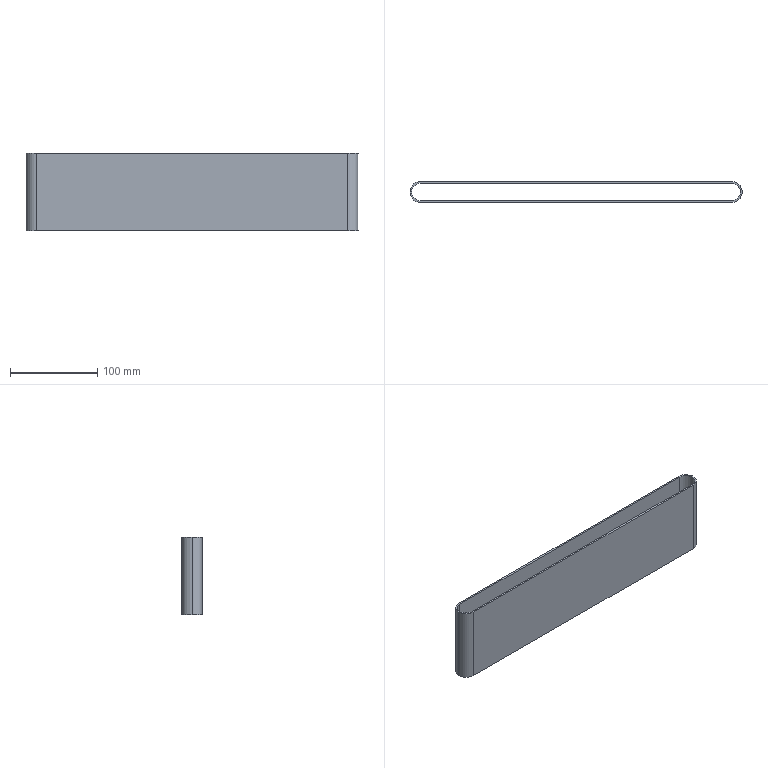Part | STEP file | Green flat belt | 1 solid | 12 faces | box 380 x 24 x 89 mm | volume 139038 mm3 | cylinder 6 | plane 6 | commonest cylinder face diameters 20 x3 24 x3
STEP:
#1=CARTESIAN_POINT('',(-176.888,10.,89.));
#2=VERTEX_POINT('',#1);
#3=CARTESIAN_POINT('',(-186.888,0.,89.));
#4=VERTEX_POINT('',#3);
#5=CARTESIAN_POINT('',(-176.888,0.,89.));
#6=DIRECTION('',(0.,0.,1.));
#7=DIRECTION('',(1.,0.,0.));
#8=AXIS2_PLACEMENT_3D('',#5,#6,#7);
#9=CIRCLE('',#8,10.);
#10=EDGE_CURVE('',#2,#4,#9,.T.);
#11=ORIENTED_EDGE('',*,*,#10,.T.);
#12=CARTESIAN_POINT('',(-186.888,0.,0.));
#13=VERTEX_POINT('',#12);
#14=CARTESIAN_POINT('',(-186.888,0.,89.));
#15=DIRECTION('',(0.,0.,-1.));
#16=VECTOR('',#15,1000.);
#17=LINE('',#14,#16);
#18=EDGE_CURVE('',#4,#13,#17,.T.);
#19=ORIENTED_EDGE('',*,*,#18,.T.);
#20=CARTESIAN_POINT('',(-176.888,10.,0.));
#21=VERTEX_POINT('',#20);
#22=CARTESIAN_POINT('',(-176.888,0.,0.));
#23=DIRECTION('',(0.,0.,1.));
#24=DIRECTION('',(1.,0.,0.));
#25=AXIS2_PLACEMENT_3D('',#22,#23,#24);
#26=CIRCLE('',#25,10.);
#27=EDGE_CURVE('',#21,#13,#26,.T.);
#28=ORIENTED_EDGE('',*,*,#27,.F.);
#29=CARTESIAN_POINT('',(-176.888,10.,89.));
#30=DIRECTION('',(0.,0.,-1.));
#31=VECTOR('',#30,1000.);
#32=LINE('',#29,#31);
#33=EDGE_CURVE('',#2,#21,#32,.T.);
#34=ORIENTED_EDGE('',*,*,#33,.F.);
#35=EDGE_LOOP('',(#11,#19,#28,#34));
#36=FACE_OUTER_BOUND('',#35,.T.);
#37=CARTESIAN_POINT('',(-176.888,0.,89.));
#38=DIRECTION('',(0.,0.,-1.));
#39=DIRECTION('',(-1.,0.,0.));
#40=AXIS2_PLACEMENT_3D('',#37,#38,#39);
#41=CYLINDRICAL_SURFACE('',#40,10.);
#42=ADVANCED_FACE('',(#36),#41,.F.);
#43=CARTESIAN_POINT('',(-188.888,0.,89.));
#44=VERTEX_POINT('',#43);
#45=CARTESIAN_POINT('',(-176.888,-12.,89.));
#46=VERTEX_POINT('',#45);
#47=CARTESIAN_POINT('',(-176.888,0.,89.));
#48=DIRECTION('',(0.,0.,1.));
#49=DIRECTION('',(1.,0.,0.));
#50=AXIS2_PLACEMENT_3D('',#47,#48,#49);
#51=CIRCLE('',#50,12.);
#52=EDGE_CURVE('',#44,#46,#51,.T.);
#53=ORIENTED_EDGE('',*,*,#52,.F.);
#54=CARTESIAN_POINT('',(-188.888,0.,0.));
#55=VERTEX_POINT('',#54);
#56=CARTESIAN_POINT('',(-188.888,0.,89.));
#57=DIRECTION('',(0.,0.,-1.));
#58=VECTOR('',#57,1000.);
#59=LINE('',#56,#58);
#60=EDGE_CURVE('',#44,#55,#59,.T.);
#61=ORIENTED_EDGE('',*,*,#60,.T.);
#62=CARTESIAN_POINT('',(-176.888,-12.,0.));
#63=VERTEX_POINT('',#62);
#64=CARTESIAN_POINT('',(-176.888,0.,0.));
#65=DIRECTION('',(0.,0.,1.));
#66=DIRECTION('',(1.,0.,0.));
#67=AXIS2_PLACEMENT_3D('',#64,#65,#66);
#68=CIRCLE('',#67,12.);
#69=EDGE_CURVE('',#55,#63,#68,.T.);
#70=ORIENTED_EDGE('',*,*,#69,.T.);
#71=CARTESIAN_POINT('',(-176.888,-12.,89.));
#72=DIRECTION('',(0.,0.,-1.));
#73=VECTOR('',#72,1000.);
#74=LINE('',#71,#73);
#75=EDGE_CURVE('',#46,#63,#74,.T.);
#76=ORIENTED_EDGE('',*,*,#75,.F.);
#77=EDGE_LOOP('',(#53,#61,#70,#76));
#78=FACE_OUTER_BOUND('',#77,.T.);
#79=CARTESIAN_POINT('',(-176.888,0.,89.));
#80=DIRECTION('',(0.,0.,-1.));
#81=DIRECTION('',(-1.,0.,0.));
#82=AXIS2_PLACEMENT_3D('',#79,#80,#81);
#83=CYLINDRICAL_SURFACE('',#82,12.);
#84=ADVANCED_FACE('',(#78),#83,.T.);
#85=CARTESIAN_POINT('',(-176.888,12.,89.));
#86=VERTEX_POINT('',#85);
#87=CARTESIAN_POINT('',(-176.888,0.,89.));
#88=DIRECTION('',(0.,0.,1.));
#89=DIRECTION('',(1.,0.,0.));
#90=AXIS2_PLACEMENT_3D('',#87,#88,#89);
#91=CIRCLE('',#90,12.);
#92=EDGE_CURVE('',#86,#44,#91,.T.);
#93=ORIENTED_EDGE('',*,*,#92,.T.);
#94=ORIENTED_EDGE('',*,*,#52,.T.);
#95=CARTESIAN_POINT('',(179.112,-12.,89.));
#96=VERTEX_POINT('',#95);
#97=CARTESIAN_POINT('',(-176.888,-12.,89.));
#98=DIRECTION('',(1.,0.,0.));
#99=VECTOR('',#98,1000.);
#100=LINE('',#97,#99);
#101=EDGE_CURVE('',#46,#96,#100,.T.);
#102=ORIENTED_EDGE('',*,*,#101,.T.);
#103=CARTESIAN_POINT('',(179.112,12.,89.));
#104=VERTEX_POINT('',#103);
#105=CARTESIAN_POINT('',(179.112,0.,89.));
#106=DIRECTION('',(0.,0.,1.));
#107=DIRECTION('',(1.,0.,0.));
#108=AXIS2_PLACEMENT_3D('',#105,#106,#107);
#109=CIRCLE('',#108,12.);
#110=EDGE_CURVE('',#96,#104,#109,.T.);
#111=ORIENTED_EDGE('',*,*,#110,.T.);
#112=CARTESIAN_POINT('',(-176.888,12.,89.));
#113=DIRECTION('',(-1.,0.,0.));
#114=VECTOR('',#113,1000.);
#115=LINE('',#112,#114);
#116=EDGE_CURVE('',#104,#86,#115,.T.);
#117=ORIENTED_EDGE('',*,*,#116,.T.);
#118=EDGE_LOOP('',(#93,#94,#102,#111,#117));
#119=FACE_OUTER_BOUND('',#118,.T.);
#120=CARTESIAN_POINT('',(-176.888,-10.,89.));
#121=VERTEX_POINT('',#120);
#122=CARTESIAN_POINT('',(179.112,-10.,89.));
#123=VERTEX_POINT('',#122);
#124=CARTESIAN_POINT('',(-176.888,-10.,89.));
#125=DIRECTION('',(1.,0.,0.));
#126=VECTOR('',#125,1000.);
#127=LINE('',#124,#126);
#128=EDGE_CURVE('',#121,#123,#127,.T.);
#129=ORIENTED_EDGE('',*,*,#128,.F.);
#130=CARTESIAN_POINT('',(-176.888,0.,89.));
#131=DIRECTION('',(0.,0.,1.));
#132=DIRECTION('',(1.,0.,0.));
#133=AXIS2_PLACEMENT_3D('',#130,#131,#132);
#134=CIRCLE('',#133,10.);
#135=EDGE_CURVE('',#4,#121,#134,.T.);
#136=ORIENTED_EDGE('',*,*,#135,.F.);
#137=ORIENTED_EDGE('',*,*,#10,.F.);
#138=CARTESIAN_POINT('',(179.112,10.,89.));
#139=VERTEX_POINT('',#138);
#140=CARTESIAN_POINT('',(-176.888,10.,89.));
#141=DIRECTION('',(-1.,0.,0.));
#142=VECTOR('',#141,1000.);
#143=LINE('',#140,#142);
#144=EDGE_CURVE('',#139,#2,#143,.T.);
#145=ORIENTED_EDGE('',*,*,#144,.F.);
#146=CARTESIAN_POINT('',(179.112,0.,89.));
#147=DIRECTION('',(0.,0.,1.));
#148=DIRECTION('',(1.,0.,0.));
#149=AXIS2_PLACEMENT_3D('',#146,#147,#148);
#150=CIRCLE('',#149,10.);
#151=EDGE_CURVE('',#123,#139,#150,.T.);
#152=ORIENTED_EDGE('',*,*,#151,.F.);
#153=EDGE_LOOP('',(#129,#136,#137,#145,#152));
#154=FACE_BOUND('',#153,.T.);
#155=CARTESIAN_POINT('',(-176.888,0.,89.));
#156=DIRECTION('',(0.,0.,1.));
#157=DIRECTION('',(1.,0.,0.));
#158=AXIS2_PLACEMENT_3D('',#155,#156,#157);
#159=PLANE('',#158);
#160=ADVANCED_FACE('',(#119,#154),#159,.T.);
#161=CARTESIAN_POINT('',(-176.888,12.,0.));
#162=VERTEX_POINT('',#161);
#163=CARTESIAN_POINT('',(-176.888,0.,0.));
#164=DIRECTION('',(0.,0.,1.));
#165=DIRECTION('',(1.,0.,0.));
#166=AXIS2_PLACEMENT_3D('',#163,#164,#165);
#167=CIRCLE('',#166,12.);
#168=EDGE_CURVE('',#162,#55,#167,.T.);
#169=ORIENTED_EDGE('',*,*,#168,.F.);
#170=CARTESIAN_POINT('',(179.112,12.,0.));
#171=VERTEX_POINT('',#170);
#172=CARTESIAN_POINT('',(-176.888,12.,0.));
#173=DIRECTION('',(-1.,0.,0.));
#174=VECTOR('',#173,1000.);
#175=LINE('',#172,#174);
#176=EDGE_CURVE('',#171,#162,#175,.T.);
#177=ORIENTED_EDGE('',*,*,#176,.F.);
#178=CARTESIAN_POINT('',(179.112,-12.,0.));
#179=VERTEX_POINT('',#178);
#180=CARTESIAN_POINT('',(179.112,0.,0.));
#181=DIRECTION('',(0.,0.,1.));
#182=DIRECTION('',(1.,0.,0.));
#183=AXIS2_PLACEMENT_3D('',#180,#181,#182);
#184=CIRCLE('',#183,12.);
#185=EDGE_CURVE('',#179,#171,#184,.T.);
#186=ORIENTED_EDGE('',*,*,#185,.F.);
#187=CARTESIAN_POINT('',(-176.888,-12.,0.));
#188=DIRECTION('',(1.,0.,0.));
#189=VECTOR('',#188,1000.);
#190=LINE('',#187,#189);
#191=EDGE_CURVE('',#63,#179,#190,.T.);
#192=ORIENTED_EDGE('',*,*,#191,.F.);
#193=ORIENTED_EDGE('',*,*,#69,.F.);
#194=EDGE_LOOP('',(#169,#177,#186,#192,#193));
#195=FACE_OUTER_BOUND('',#194,.T.);
#196=ORIENTED_EDGE('',*,*,#27,.T.);
#197=CARTESIAN_POINT('',(-176.888,-10.,0.));
#198=VERTEX_POINT('',#197);
#199=CARTESIAN_POINT('',(-176.888,0.,0.));
#200=DIRECTION('',(0.,0.,1.));
#201=DIRECTION('',(1.,0.,0.));
#202=AXIS2_PLACEMENT_3D('',#199,#200,#201);
#203=CIRCLE('',#202,10.);
#204=EDGE_CURVE('',#13,#198,#203,.T.);
#205=ORIENTED_EDGE('',*,*,#204,.T.);
#206=CARTESIAN_POINT('',(179.112,-10.,0.));
#207=VERTEX_POINT('',#206);
#208=CARTESIAN_POINT('',(-176.888,-10.,0.));
#209=DIRECTION('',(1.,0.,0.));
#210=VECTOR('',#209,1000.);
#211=LINE('',#208,#210);
#212=EDGE_CURVE('',#198,#207,#211,.T.);
#213=ORIENTED_EDGE('',*,*,#212,.T.);
#214=CARTESIAN_POINT('',(179.112,10.,0.));
#215=VERTEX_POINT('',#214);
#216=CARTESIAN_POINT('',(179.112,0.,0.));
#217=DIRECTION('',(0.,0.,1.));
#218=DIRECTION('',(1.,0.,0.));
#219=AXIS2_PLACEMENT_3D('',#216,#217,#218);
#220=CIRCLE('',#219,10.);
#221=EDGE_CURVE('',#207,#215,#220,.T.);
#222=ORIENTED_EDGE('',*,*,#221,.T.);
#223=CARTESIAN_POINT('',(-176.888,10.,0.));
#224=DIRECTION('',(-1.,0.,0.));
#225=VECTOR('',#224,1000.);
#226=LINE('',#223,#225);
#227=EDGE_CURVE('',#215,#21,#226,.T.);
#228=ORIENTED_EDGE('',*,*,#227,.T.);
#229=EDGE_LOOP('',(#196,#205,#213,#222,#228));
#230=FACE_BOUND('',#229,.T.);
#231=CARTESIAN_POINT('',(-176.888,0.,0.));
#232=DIRECTION('',(0.,0.,1.));
#233=DIRECTION('',(1.,0.,0.));
#234=AXIS2_PLACEMENT_3D('',#231,#232,#233);
#235=PLANE('',#234);
#236=ADVANCED_FACE('',(#195,#230),#235,.F.);
#237=ORIENTED_EDGE('',*,*,#60,.F.);
#238=ORIENTED_EDGE('',*,*,#92,.F.);
#239=CARTESIAN_POINT('',(-176.888,12.,89.));
#240=DIRECTION('',(0.,0.,-1.));
#241=VECTOR('',#240,1000.);
#242=LINE('',#239,#241);
#243=EDGE_CURVE('',#86,#162,#242,.T.);
#244=ORIENTED_EDGE('',*,*,#243,.T.);
#245=ORIENTED_EDGE('',*,*,#168,.T.);
#246=EDGE_LOOP('',(#237,#238,#244,#245));
#247=FACE_OUTER_BOUND('',#246,.T.);
#248=CARTESIAN_POINT('',(-176.888,0.,89.));
#249=DIRECTION('',(0.,0.,-1.));
#250=DIRECTION('',(-1.,0.,0.));
#251=AXIS2_PLACEMENT_3D('',#248,#249,#250);
#252=CYLINDRICAL_SURFACE('',#251,12.);
#253=ADVANCED_FACE('',(#247),#252,.T.);
#254=ORIENTED_EDGE('',*,*,#191,.T.);
#255=CARTESIAN_POINT('',(179.112,-12.,89.));
#256=DIRECTION('',(0.,0.,-1.));
#257=VECTOR('',#256,1000.);
#258=LINE('',#255,#257);
#259=EDGE_CURVE('',#96,#179,#258,.T.);
#260=ORIENTED_EDGE('',*,*,#259,.F.);
#261=ORIENTED_EDGE('',*,*,#101,.F.);
#262=ORIENTED_EDGE('',*,*,#75,.T.);
#263=EDGE_LOOP('',(#254,#260,#261,#262));
#264=FACE_OUTER_BOUND('',#263,.T.);
#265=CARTESIAN_POINT('',(-176.888,-12.,89.));
#266=DIRECTION('',(0.,1.,0.));
#267=DIRECTION('',(0.,0.,1.));
#268=AXIS2_PLACEMENT_3D('',#265,#266,#267);
#269=PLANE('',#268);
#270=ADVANCED_FACE('',(#264),#269,.F.);
#271=ORIENTED_EDGE('',*,*,#185,.T.);
#272=CARTESIAN_POINT('',(179.112,12.,89.));
#273=DIRECTION('',(0.,0.,-1.));
#274=VECTOR('',#273,1000.);
#275=LINE('',#272,#274);
#276=EDGE_CURVE('',#104,#171,#275,.T.);
#277=ORIENTED_EDGE('',*,*,#276,.F.);
#278=ORIENTED_EDGE('',*,*,#110,.F.);
#279=ORIENTED_EDGE('',*,*,#259,.T.);
#280=EDGE_LOOP('',(#271,#277,#278,#279));
#281=FACE_OUTER_BOUND('',#280,.T.);
#282=CARTESIAN_POINT('',(179.112,0.,89.));
#283=DIRECTION('',(0.,0.,-1.));
#284=DIRECTION('',(-1.,0.,0.));
#285=AXIS2_PLACEMENT_3D('',#282,#283,#284);
#286=CYLINDRICAL_SURFACE('',#285,12.);
#287=ADVANCED_FACE('',(#281),#286,.T.);
#288=ORIENTED_EDGE('',*,*,#176,.T.);
#289=ORIENTED_EDGE('',*,*,#243,.F.);
#290=ORIENTED_EDGE('',*,*,#116,.F.);
#291=ORIENTED_EDGE('',*,*,#276,.T.);
#292=EDGE_LOOP('',(#288,#289,#290,#291));
#293=FACE_OUTER_BOUND('',#292,.T.);
#294=CARTESIAN_POINT('',(-176.888,12.,89.));
#295=DIRECTION('',(0.,-1.,0.));
#296=DIRECTION('',(0.,0.,-1.));
#297=AXIS2_PLACEMENT_3D('',#294,#295,#296);
#298=PLANE('',#297);
#299=ADVANCED_FACE('',(#293),#298,.F.);
#300=ORIENTED_EDGE('',*,*,#18,.F.);
#301=ORIENTED_EDGE('',*,*,#135,.T.);
#302=CARTESIAN_POINT('',(-176.888,-10.,89.));
#303=DIRECTION('',(0.,0.,-1.));
#304=VECTOR('',#303,1000.);
#305=LINE('',#302,#304);
#306=EDGE_CURVE('',#121,#198,#305,.T.);
#307=ORIENTED_EDGE('',*,*,#306,.T.);
#308=ORIENTED_EDGE('',*,*,#204,.F.);
#309=EDGE_LOOP('',(#300,#301,#307,#308));
#310=FACE_OUTER_BOUND('',#309,.T.);
#311=CARTESIAN_POINT('',(-176.888,0.,89.));
#312=DIRECTION('',(0.,0.,-1.));
#313=DIRECTION('',(-1.,0.,0.));
#314=AXIS2_PLACEMENT_3D('',#311,#312,#313);
#315=CYLINDRICAL_SURFACE('',#314,10.);
#316=ADVANCED_FACE('',(#310),#315,.F.);
#317=ORIENTED_EDGE('',*,*,#212,.F.);
#318=ORIENTED_EDGE('',*,*,#306,.F.);
#319=ORIENTED_EDGE('',*,*,#128,.T.);
#320=CARTESIAN_POINT('',(179.112,-10.,89.));
#321=DIRECTION('',(0.,0.,-1.));
#322=VECTOR('',#321,1000.);
#323=LINE('',#320,#322);
#324=EDGE_CURVE('',#123,#207,#323,.T.);
#325=ORIENTED_EDGE('',*,*,#324,.T.);
#326=EDGE_LOOP('',(#317,#318,#319,#325));
#327=FACE_OUTER_BOUND('',#326,.T.);
#328=CARTESIAN_POINT('',(-176.888,-10.,89.));
#329=DIRECTION('',(0.,1.,0.));
#330=DIRECTION('',(-1.,0.,0.));
#331=AXIS2_PLACEMENT_3D('',#328,#329,#330);
#332=PLANE('',#331);
#333=ADVANCED_FACE('',(#327),#332,.T.);
#334=ORIENTED_EDGE('',*,*,#221,.F.);
#335=ORIENTED_EDGE('',*,*,#324,.F.);
#336=ORIENTED_EDGE('',*,*,#151,.T.);
#337=CARTESIAN_POINT('',(179.112,10.,89.));
#338=DIRECTION('',(0.,0.,-1.));
#339=VECTOR('',#338,1000.);
#340=LINE('',#337,#339);
#341=EDGE_CURVE('',#139,#215,#340,.T.);
#342=ORIENTED_EDGE('',*,*,#341,.T.);
#343=EDGE_LOOP('',(#334,#335,#336,#342));
#344=FACE_OUTER_BOUND('',#343,.T.);
#345=CARTESIAN_POINT('',(179.112,0.,89.));
#346=DIRECTION('',(0.,0.,-1.));
#347=DIRECTION('',(-1.,0.,0.));
#348=AXIS2_PLACEMENT_3D('',#345,#346,#347);
#349=CYLINDRICAL_SURFACE('',#348,10.);
#350=ADVANCED_FACE('',(#344),#349,.F.);
#351=ORIENTED_EDGE('',*,*,#227,.F.);
#352=ORIENTED_EDGE('',*,*,#341,.F.);
#353=ORIENTED_EDGE('',*,*,#144,.T.);
#354=ORIENTED_EDGE('',*,*,#33,.T.);
#355=EDGE_LOOP('',(#351,#352,#353,#354));
#356=FACE_OUTER_BOUND('',#355,.T.);
#357=CARTESIAN_POINT('',(-176.888,10.,89.));
#358=DIRECTION('',(0.,-1.,0.));
#359=DIRECTION('',(1.,0.,0.));
#360=AXIS2_PLACEMENT_3D('',#357,#358,#359);
#361=PLANE('',#360);
#362=ADVANCED_FACE('',(#356),#361,.T.);
#363=CLOSED_SHELL('',(#42,#84,#160,#236,#253,#270,#287,#299,#316,#333,#350,#362));
#364=MANIFOLD_SOLID_BREP('',#363);
#365=CARTESIAN_POINT('',(0.,0.,0.));
#366=DIRECTION('',(0.,0.,1.));
#367=DIRECTION('',(1.,0.,0.));
#368=AXIS2_PLACEMENT_3D('',#365,#366,#367);
#369=(LENGTH_UNIT()NAMED_UNIT(*)SI_UNIT(.MILLI.,.METRE.));
#370=UNCERTAINTY_MEASURE_WITH_UNIT(LENGTH_MEASURE(0.00001),#369,'','');
#371=(NAMED_UNIT(*)PLANE_ANGLE_UNIT()SI_UNIT($,.RADIAN.));
#372=(NAMED_UNIT(*)SI_UNIT($,.STERADIAN.)SOLID_ANGLE_UNIT());
#373=(GEOMETRIC_REPRESENTATION_CONTEXT(3)GLOBAL_UNCERTAINTY_ASSIGNED_CONTEXT((#370))GLOBAL_UNIT_ASSIGNED_CONTEXT((#369,#371,#372))REPRESENTATION_CONTEXT('',''));
#374=ADVANCED_BREP_SHAPE_REPRESENTATION('',(#364,#368),#373);